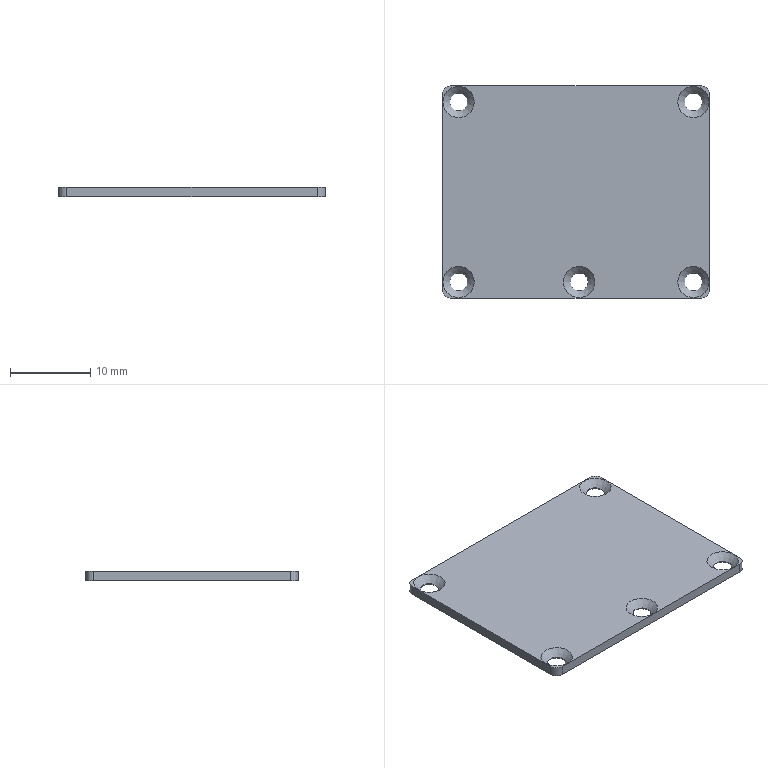Part | STEP file | 1 to 2 power divider cover | 1 solid | 25 faces | box 33.2 x 26.38 x 1.2 mm | volume 1010 mm3 | cone 10 | cylinder 9 | plane 6 | commonest cylinder face diameters 2.2 x5 2 x4